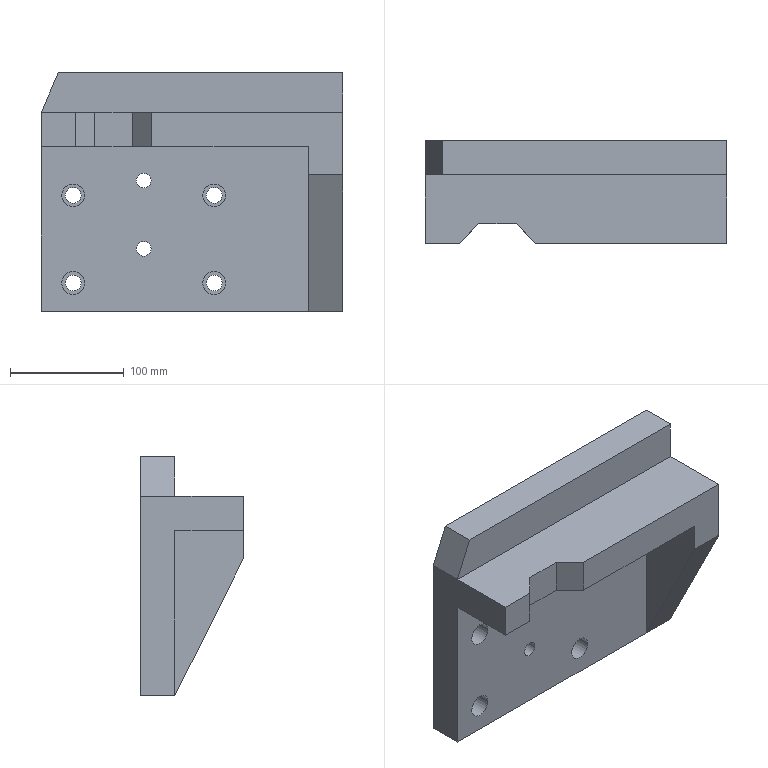Part | NX | features solid 2 | 1 solid | 31 faces | box 265 x 90 x 210 mm | volume 2230075 mm3 | plane 21 | cylinder 10 | commonest cylinder face diameters 14 x4 20 x4 13 x2
STEP:
#1=CARTESIAN_POINT('',(40.,505.,-125.));
#2=VERTEX_POINT('',#1);
#3=CARTESIAN_POINT('',(70.,505.,-125.));
#4=VERTEX_POINT('',#3);
#5=CARTESIAN_POINT('',(40.,505.,-125.));
#6=DIRECTION('',(1.,0.,0.));
#7=VECTOR('',#6,1000.);
#8=LINE('',#5,#7);
#9=EDGE_CURVE('',#2,#4,#8,.T.);
#10=ORIENTED_EDGE('',*,*,#9,.T.);
#11=CARTESIAN_POINT('',(70.,505.,-70.));
#12=VERTEX_POINT('',#11);
#13=CARTESIAN_POINT('',(70.,505.,-70.));
#14=DIRECTION('',(0.,0.,-1.));
#15=VECTOR('',#14,1000.);
#16=LINE('',#13,#15);
#17=EDGE_CURVE('',#12,#4,#16,.T.);
#18=ORIENTED_EDGE('',*,*,#17,.F.);
#19=CARTESIAN_POINT('',(-98.,505.,-70.));
#20=VERTEX_POINT('',#19);
#21=CARTESIAN_POINT('',(-235.,505.,-70.));
#22=DIRECTION('',(-1.,0.,0.));
#23=VECTOR('',#22,1000.);
#24=LINE('',#21,#23);
#25=EDGE_CURVE('',#20,#12,#24,.F.);
#26=ORIENTED_EDGE('',*,*,#25,.F.);
#27=CARTESIAN_POINT('',(-98.,505.,-100.));
#28=VERTEX_POINT('',#27);
#29=CARTESIAN_POINT('',(-98.,505.,-95.974));
#30=DIRECTION('',(0.,0.,-1.));
#31=VECTOR('',#30,1000.);
#32=LINE('',#29,#31);
#33=EDGE_CURVE('',#20,#28,#32,.T.);
#34=ORIENTED_EDGE('',*,*,#33,.T.);
#35=CARTESIAN_POINT('',(40.,505.,-100.));
#36=VERTEX_POINT('',#35);
#37=CARTESIAN_POINT('',(70.,505.,-100.));
#38=DIRECTION('',(-1.,0.,0.));
#39=VECTOR('',#38,1000.);
#40=LINE('',#37,#39);
#41=EDGE_CURVE('',#28,#36,#40,.F.);
#42=ORIENTED_EDGE('',*,*,#41,.T.);
#43=CARTESIAN_POINT('',(40.,505.,-95.974));
#44=DIRECTION('',(0.,0.,-1.));
#45=VECTOR('',#44,1000.);
#46=LINE('',#43,#45);
#47=EDGE_CURVE('',#36,#2,#46,.T.);
#48=ORIENTED_EDGE('',*,*,#47,.T.);
#49=EDGE_LOOP('',(#10,#18,#26,#34,#42,#48));
#50=FACE_BOUND('',#49,.T.);
#51=CARTESIAN_POINT('',(115.,505.,-95.974));
#52=DIRECTION('',(0.,1.,0.));
#53=DIRECTION('',(-1.,0.,0.));
#54=AXIS2_PLACEMENT_3D('',#51,#52,#53);
#55=PLANE('',#54);
#56=ADVANCED_FACE('',(#50),#55,.F.);
#57=CARTESIAN_POINT('',(-50.,595.,-143.));
#58=VERTEX_POINT('',#57);
#59=CARTESIAN_POINT('',(-43.,595.,-143.));
#60=DIRECTION('',(0.,1.,0.));
#61=DIRECTION('',(-1.,0.,0.));
#62=AXIS2_PLACEMENT_3D('',#59,#60,#61);
#63=CIRCLE('',#62,7.);
#64=EDGE_CURVE('',#58,#58,#63,.F.);
#65=ORIENTED_EDGE('',*,*,#64,.T.);
#66=EDGE_LOOP('',(#65));
#67=FACE_BOUND('',#66,.T.);
#68=CARTESIAN_POINT('',(-111.5,595.,-130.));
#69=VERTEX_POINT('',#68);
#70=CARTESIAN_POINT('',(-105.,595.,-130.));
#71=DIRECTION('',(0.,1.,0.));
#72=DIRECTION('',(-1.,0.,0.));
#73=AXIS2_PLACEMENT_3D('',#70,#71,#72);
#74=CIRCLE('',#73,6.5);
#75=EDGE_CURVE('',#69,#69,#74,.T.);
#76=ORIENTED_EDGE('',*,*,#75,.F.);
#77=EDGE_LOOP('',(#76));
#78=FACE_BOUND('',#77,.T.);
#79=CARTESIAN_POINT('',(-50.,595.,-220.));
#80=VERTEX_POINT('',#79);
#81=CARTESIAN_POINT('',(-43.,595.,-220.));
#82=DIRECTION('',(0.,1.,0.));
#83=DIRECTION('',(-1.,0.,0.));
#84=AXIS2_PLACEMENT_3D('',#81,#82,#83);
#85=CIRCLE('',#84,7.);
#86=EDGE_CURVE('',#80,#80,#85,.F.);
#87=ORIENTED_EDGE('',*,*,#86,.T.);
#88=EDGE_LOOP('',(#87));
#89=FACE_BOUND('',#88,.T.);
#90=CARTESIAN_POINT('',(-111.5,595.,-190.));
#91=VERTEX_POINT('',#90);
#92=CARTESIAN_POINT('',(-105.,595.,-190.));
#93=DIRECTION('',(0.,1.,0.));
#94=DIRECTION('',(-1.,0.,0.));
#95=AXIS2_PLACEMENT_3D('',#92,#93,#94);
#96=CIRCLE('',#95,6.5);
#97=EDGE_CURVE('',#91,#91,#96,.T.);
#98=ORIENTED_EDGE('',*,*,#97,.F.);
#99=EDGE_LOOP('',(#98));
#100=FACE_BOUND('',#99,.T.);
#101=CARTESIAN_POINT('',(-174.,595.,-220.));
#102=VERTEX_POINT('',#101);
#103=CARTESIAN_POINT('',(-167.,595.,-220.));
#104=DIRECTION('',(0.,1.,0.));
#105=DIRECTION('',(-1.,0.,0.));
#106=AXIS2_PLACEMENT_3D('',#103,#104,#105);
#107=CIRCLE('',#106,7.);
#108=EDGE_CURVE('',#102,#102,#107,.F.);
#109=ORIENTED_EDGE('',*,*,#108,.T.);
#110=EDGE_LOOP('',(#109));
#111=FACE_BOUND('',#110,.T.);
#112=CARTESIAN_POINT('',(-174.,595.,-143.));
#113=VERTEX_POINT('',#112);
#114=CARTESIAN_POINT('',(-167.,595.,-143.));
#115=DIRECTION('',(0.,1.,0.));
#116=DIRECTION('',(-1.,0.,0.));
#117=AXIS2_PLACEMENT_3D('',#114,#115,#116);
#118=CIRCLE('',#117,7.);
#119=EDGE_CURVE('',#113,#113,#118,.F.);
#120=ORIENTED_EDGE('',*,*,#119,.T.);
#121=EDGE_LOOP('',(#120));
#122=FACE_BOUND('',#121,.T.);
#123=CARTESIAN_POINT('',(-180.,595.,-35.));
#124=VERTEX_POINT('',#123);
#125=CARTESIAN_POINT('',(70.,595.,-35.));
#126=VERTEX_POINT('',#125);
#127=CARTESIAN_POINT('',(-70.,595.,-35.));
#128=DIRECTION('',(-1.,0.,0.));
#129=VECTOR('',#128,1000.);
#130=LINE('',#127,#129);
#131=EDGE_CURVE('',#124,#126,#130,.F.);
#132=ORIENTED_EDGE('',*,*,#131,.T.);
#133=CARTESIAN_POINT('',(70.,595.,-245.));
#134=VERTEX_POINT('',#133);
#135=CARTESIAN_POINT('',(70.,595.,-55.974));
#136=DIRECTION('',(0.,0.,-1.));
#137=VECTOR('',#136,1000.);
#138=LINE('',#135,#137);
#139=EDGE_CURVE('',#126,#134,#138,.T.);
#140=ORIENTED_EDGE('',*,*,#139,.T.);
#141=CARTESIAN_POINT('',(-195.,595.,-245.));
#142=VERTEX_POINT('',#141);
#143=CARTESIAN_POINT('',(-195.,595.,-245.));
#144=DIRECTION('',(-1.,0.,0.));
#145=VECTOR('',#144,1000.);
#146=LINE('',#143,#145);
#147=EDGE_CURVE('',#142,#134,#146,.F.);
#148=ORIENTED_EDGE('',*,*,#147,.F.);
#149=CARTESIAN_POINT('',(-195.,595.,-70.));
#150=VERTEX_POINT('',#149);
#151=CARTESIAN_POINT('',(-195.,595.,-245.));
#152=DIRECTION('',(0.,0.,1.));
#153=VECTOR('',#152,1000.);
#154=LINE('',#151,#153);
#155=EDGE_CURVE('',#150,#142,#154,.F.);
#156=ORIENTED_EDGE('',*,*,#155,.F.);
#157=CARTESIAN_POINT('',(-141.818,595.,54.091));
#158=DIRECTION('',(-0.3939,0.,-0.9191));
#159=VECTOR('',#158,1000.);
#160=LINE('',#157,#159);
#161=EDGE_CURVE('',#150,#124,#160,.F.);
#162=ORIENTED_EDGE('',*,*,#161,.T.);
#163=EDGE_LOOP('',(#132,#140,#148,#156,#162));
#164=FACE_BOUND('',#163,.T.);
#165=CARTESIAN_POINT('',(115.,595.,-55.974));
#166=DIRECTION('',(0.,1.,0.));
#167=DIRECTION('',(-1.,0.,0.));
#168=AXIS2_PLACEMENT_3D('',#165,#166,#167);
#169=PLANE('',#168);
#170=ADVANCED_FACE('',(#67,#78,#89,#100,#111,#122,#164),#169,.T.);
#171=ORIENTED_EDGE('',*,*,#147,.T.);
#172=CARTESIAN_POINT('',(70.,565.,-245.));
#173=VERTEX_POINT('',#172);
#174=CARTESIAN_POINT('',(70.,595.,-245.));
#175=DIRECTION('',(0.,-1.,0.));
#176=VECTOR('',#175,1000.);
#177=LINE('',#174,#176);
#178=EDGE_CURVE('',#134,#173,#177,.T.);
#179=ORIENTED_EDGE('',*,*,#178,.T.);
#180=CARTESIAN_POINT('',(40.,565.,-245.));
#181=VERTEX_POINT('',#180);
#182=CARTESIAN_POINT('',(-195.,565.,-245.));
#183=DIRECTION('',(1.,0.,0.));
#184=VECTOR('',#183,1000.);
#185=LINE('',#182,#184);
#186=EDGE_CURVE('',#181,#173,#185,.T.);
#187=ORIENTED_EDGE('',*,*,#186,.F.);
#188=CARTESIAN_POINT('',(-195.,565.,-245.));
#189=VERTEX_POINT('',#188);
#190=CARTESIAN_POINT('',(-195.,565.,-245.));
#191=DIRECTION('',(-1.,0.,0.));
#192=VECTOR('',#191,1000.);
#193=LINE('',#190,#192);
#194=EDGE_CURVE('',#189,#181,#193,.F.);
#195=ORIENTED_EDGE('',*,*,#194,.F.);
#196=CARTESIAN_POINT('',(-195.,595.,-245.));
#197=DIRECTION('',(0.,-1.,0.));
#198=VECTOR('',#197,1000.);
#199=LINE('',#196,#198);
#200=EDGE_CURVE('',#142,#189,#199,.T.);
#201=ORIENTED_EDGE('',*,*,#200,.F.);
#202=EDGE_LOOP('',(#171,#179,#187,#195,#201));
#203=FACE_BOUND('',#202,.T.);
#204=CARTESIAN_POINT('',(-195.,595.,-245.));
#205=DIRECTION('',(0.,0.,-1.));
#206=DIRECTION('',(0.,-1.,0.));
#207=AXIS2_PLACEMENT_3D('',#204,#205,#206);
#208=PLANE('',#207);
#209=ADVANCED_FACE('',(#203),#208,.T.);
#210=CARTESIAN_POINT('',(-43.,565.,-210.));
#211=VERTEX_POINT('',#210);
#212=CARTESIAN_POINT('',(-43.,565.,-220.));
#213=DIRECTION('',(0.,1.,0.));
#214=DIRECTION('',(0.,0.,1.));
#215=AXIS2_PLACEMENT_3D('',#212,#213,#214);
#216=CIRCLE('',#215,10.);
#217=EDGE_CURVE('',#211,#211,#216,.T.);
#218=ORIENTED_EDGE('',*,*,#217,.T.);
#219=EDGE_LOOP('',(#218));
#220=FACE_BOUND('',#219,.T.);
#221=CARTESIAN_POINT('',(-43.,565.,-133.));
#222=VERTEX_POINT('',#221);
#223=CARTESIAN_POINT('',(-43.,565.,-143.));
#224=DIRECTION('',(0.,1.,0.));
#225=DIRECTION('',(0.,0.,1.));
#226=AXIS2_PLACEMENT_3D('',#223,#224,#225);
#227=CIRCLE('',#226,10.);
#228=EDGE_CURVE('',#222,#222,#227,.T.);
#229=ORIENTED_EDGE('',*,*,#228,.T.);
#230=EDGE_LOOP('',(#229));
#231=FACE_BOUND('',#230,.T.);
#232=CARTESIAN_POINT('',(-167.,565.,-133.));
#233=VERTEX_POINT('',#232);
#234=CARTESIAN_POINT('',(-167.,565.,-143.));
#235=DIRECTION('',(0.,1.,0.));
#236=DIRECTION('',(0.,0.,1.));
#237=AXIS2_PLACEMENT_3D('',#234,#235,#236);
#238=CIRCLE('',#237,10.);
#239=EDGE_CURVE('',#233,#233,#238,.T.);
#240=ORIENTED_EDGE('',*,*,#239,.T.);
#241=EDGE_LOOP('',(#240));
#242=FACE_BOUND('',#241,.T.);
#243=CARTESIAN_POINT('',(-167.,565.,-210.));
#244=VERTEX_POINT('',#243);
#245=CARTESIAN_POINT('',(-167.,565.,-220.));
#246=DIRECTION('',(0.,1.,0.));
#247=DIRECTION('',(0.,0.,1.));
#248=AXIS2_PLACEMENT_3D('',#245,#246,#247);
#249=CIRCLE('',#248,10.);
#250=EDGE_CURVE('',#244,#244,#249,.T.);
#251=ORIENTED_EDGE('',*,*,#250,.T.);
#252=EDGE_LOOP('',(#251));
#253=FACE_BOUND('',#252,.T.);
#254=CARTESIAN_POINT('',(-111.5,565.,-190.));
#255=VERTEX_POINT('',#254);
#256=CARTESIAN_POINT('',(-105.,565.,-190.));
#257=DIRECTION('',(0.,1.,0.));
#258=DIRECTION('',(-1.,0.,0.));
#259=AXIS2_PLACEMENT_3D('',#256,#257,#258);
#260=CIRCLE('',#259,6.5);
#261=EDGE_CURVE('',#255,#255,#260,.T.);
#262=ORIENTED_EDGE('',*,*,#261,.T.);
#263=EDGE_LOOP('',(#262));
#264=FACE_BOUND('',#263,.T.);
#265=CARTESIAN_POINT('',(-111.5,565.,-130.));
#266=VERTEX_POINT('',#265);
#267=CARTESIAN_POINT('',(-105.,565.,-130.));
#268=DIRECTION('',(0.,1.,0.));
#269=DIRECTION('',(-1.,0.,0.));
#270=AXIS2_PLACEMENT_3D('',#267,#268,#269);
#271=CIRCLE('',#270,6.5);
#272=EDGE_CURVE('',#266,#266,#271,.T.);
#273=ORIENTED_EDGE('',*,*,#272,.T.);
#274=EDGE_LOOP('',(#273));
#275=FACE_BOUND('',#274,.T.);
#276=ORIENTED_EDGE('',*,*,#194,.T.);
#277=CARTESIAN_POINT('',(40.,565.,-100.));
#278=VERTEX_POINT('',#277);
#279=CARTESIAN_POINT('',(40.,565.,-55.974));
#280=DIRECTION('',(0.,0.,-1.));
#281=VECTOR('',#280,1000.);
#282=LINE('',#279,#281);
#283=EDGE_CURVE('',#278,#181,#282,.T.);
#284=ORIENTED_EDGE('',*,*,#283,.F.);
#285=CARTESIAN_POINT('',(-195.,565.,-100.));
#286=VERTEX_POINT('',#285);
#287=CARTESIAN_POINT('',(70.,565.,-100.));
#288=DIRECTION('',(-1.,0.,0.));
#289=VECTOR('',#288,1000.);
#290=LINE('',#287,#289);
#291=EDGE_CURVE('',#286,#278,#290,.F.);
#292=ORIENTED_EDGE('',*,*,#291,.F.);
#293=CARTESIAN_POINT('',(-195.,565.,-245.));
#294=DIRECTION('',(0.,0.,1.));
#295=VECTOR('',#294,1000.);
#296=LINE('',#293,#295);
#297=EDGE_CURVE('',#286,#189,#296,.F.);
#298=ORIENTED_EDGE('',*,*,#297,.T.);
#299=EDGE_LOOP('',(#276,#284,#292,#298));
#300=FACE_BOUND('',#299,.T.);
#301=CARTESIAN_POINT('',(115.,565.,-55.974));
#302=DIRECTION('',(0.,1.,0.));
#303=DIRECTION('',(-1.,0.,0.));
#304=AXIS2_PLACEMENT_3D('',#301,#302,#303);
#305=PLANE('',#304);
#306=ADVANCED_FACE('',(#220,#231,#242,#253,#264,#275,#300),#305,.F.);
#307=ORIENTED_EDGE('',*,*,#200,.T.);
#308=ORIENTED_EDGE('',*,*,#297,.F.);
#309=CARTESIAN_POINT('',(-195.,505.,-100.));
#310=VERTEX_POINT('',#309);
#311=CARTESIAN_POINT('',(-195.,575.,-100.));
#312=DIRECTION('',(0.,-1.,0.));
#313=VECTOR('',#312,1000.);
#314=LINE('',#311,#313);
#315=EDGE_CURVE('',#286,#310,#314,.T.);
#316=ORIENTED_EDGE('',*,*,#315,.T.);
#317=CARTESIAN_POINT('',(-195.,505.,-70.));
#318=VERTEX_POINT('',#317);
#319=CARTESIAN_POINT('',(-195.,505.,-245.));
#320=DIRECTION('',(0.,0.,-1.));
#321=VECTOR('',#320,1000.);
#322=LINE('',#319,#321);
#323=EDGE_CURVE('',#318,#310,#322,.T.);
#324=ORIENTED_EDGE('',*,*,#323,.F.);
#325=CARTESIAN_POINT('',(-195.,565.,-70.));
#326=VERTEX_POINT('',#325);
#327=CARTESIAN_POINT('',(-195.,565.,-70.));
#328=DIRECTION('',(0.,-1.,0.));
#329=VECTOR('',#328,1000.);
#330=LINE('',#327,#329);
#331=EDGE_CURVE('',#326,#318,#330,.T.);
#332=ORIENTED_EDGE('',*,*,#331,.F.);
#333=CARTESIAN_POINT('',(-195.,615.,-70.));
#334=DIRECTION('',(0.,-1.,0.));
#335=VECTOR('',#334,1000.);
#336=LINE('',#333,#335);
#337=EDGE_CURVE('',#326,#150,#336,.F.);
#338=ORIENTED_EDGE('',*,*,#337,.T.);
#339=ORIENTED_EDGE('',*,*,#155,.T.);
#340=EDGE_LOOP('',(#307,#308,#316,#324,#332,#338,#339));
#341=FACE_BOUND('',#340,.T.);
#342=CARTESIAN_POINT('',(-195.,615.,-245.));
#343=DIRECTION('',(-1.,0.,0.));
#344=DIRECTION('',(0.,0.,1.));
#345=AXIS2_PLACEMENT_3D('',#342,#343,#344);
#346=PLANE('',#345);
#347=ADVANCED_FACE('',(#341),#346,.T.);
#348=CARTESIAN_POINT('',(-165.,505.,-100.));
#349=VERTEX_POINT('',#348);
#350=CARTESIAN_POINT('',(70.,505.,-100.));
#351=DIRECTION('',(-1.,0.,0.));
#352=VECTOR('',#351,1000.);
#353=LINE('',#350,#352);
#354=EDGE_CURVE('',#310,#349,#353,.F.);
#355=ORIENTED_EDGE('',*,*,#354,.T.);
#356=CARTESIAN_POINT('',(-165.,505.,-70.));
#357=VERTEX_POINT('',#356);
#358=CARTESIAN_POINT('',(-165.,505.,-95.974));
#359=DIRECTION('',(0.,0.,1.));
#360=VECTOR('',#359,1000.);
#361=LINE('',#358,#360);
#362=EDGE_CURVE('',#349,#357,#361,.T.);
#363=ORIENTED_EDGE('',*,*,#362,.T.);
#364=CARTESIAN_POINT('',(-235.,505.,-70.));
#365=DIRECTION('',(-1.,0.,0.));
#366=VECTOR('',#365,1000.);
#367=LINE('',#364,#366);
#368=EDGE_CURVE('',#318,#357,#367,.F.);
#369=ORIENTED_EDGE('',*,*,#368,.F.);
#370=ORIENTED_EDGE('',*,*,#323,.T.);
#371=EDGE_LOOP('',(#355,#363,#369,#370));
#372=FACE_BOUND('',#371,.T.);
#373=CARTESIAN_POINT('',(115.,505.,-95.974));
#374=DIRECTION('',(0.,1.,0.));
#375=DIRECTION('',(-1.,0.,0.));
#376=AXIS2_PLACEMENT_3D('',#373,#374,#375);
#377=PLANE('',#376);
#378=ADVANCED_FACE('',(#372),#377,.F.);
#379=CARTESIAN_POINT('',(-180.,565.,-35.));
#380=VERTEX_POINT('',#379);
#381=CARTESIAN_POINT('',(70.,565.,-35.));
#382=VERTEX_POINT('',#381);
#383=CARTESIAN_POINT('',(-70.,565.,-35.));
#384=DIRECTION('',(-1.,0.,0.));
#385=VECTOR('',#384,1000.);
#386=LINE('',#383,#385);
#387=EDGE_CURVE('',#380,#382,#386,.F.);
#388=ORIENTED_EDGE('',*,*,#387,.F.);
#389=CARTESIAN_POINT('',(-195.,565.,-70.));
#390=DIRECTION('',(0.3939,0.,0.9191));
#391=VECTOR('',#390,1000.);
#392=LINE('',#389,#391);
#393=EDGE_CURVE('',#380,#326,#392,.F.);
#394=ORIENTED_EDGE('',*,*,#393,.T.);
#395=CARTESIAN_POINT('',(70.,565.,-70.));
#396=VERTEX_POINT('',#395);
#397=CARTESIAN_POINT('',(-235.,565.,-70.));
#398=DIRECTION('',(-1.,0.,0.));
#399=VECTOR('',#398,1000.);
#400=LINE('',#397,#399);
#401=EDGE_CURVE('',#326,#396,#400,.F.);
#402=ORIENTED_EDGE('',*,*,#401,.T.);
#403=CARTESIAN_POINT('',(70.,565.,-100.));
#404=DIRECTION('',(0.,0.,1.));
#405=VECTOR('',#404,1000.);
#406=LINE('',#403,#405);
#407=EDGE_CURVE('',#396,#382,#406,.T.);
#408=ORIENTED_EDGE('',*,*,#407,.T.);
#409=EDGE_LOOP('',(#388,#394,#402,#408));
#410=FACE_BOUND('',#409,.T.);
#411=CARTESIAN_POINT('',(115.,565.,-55.974));
#412=DIRECTION('',(0.,1.,0.));
#413=DIRECTION('',(-1.,0.,0.));
#414=AXIS2_PLACEMENT_3D('',#411,#412,#413);
#415=PLANE('',#414);
#416=ADVANCED_FACE('',(#410),#415,.F.);
#417=CARTESIAN_POINT('',(-174.,580.,-220.));
#418=VERTEX_POINT('',#417);
#419=CARTESIAN_POINT('',(-167.,580.,-220.));
#420=DIRECTION('',(0.,1.,0.));
#421=DIRECTION('',(-1.,0.,0.));
#422=AXIS2_PLACEMENT_3D('',#419,#420,#421);
#423=CIRCLE('',#422,7.);
#424=EDGE_CURVE('',#418,#418,#423,.T.);
#425=ORIENTED_EDGE('',*,*,#424,.F.);
#426=EDGE_LOOP('',(#425));
#427=FACE_BOUND('',#426,.T.);
#428=ORIENTED_EDGE('',*,*,#108,.F.);
#429=EDGE_LOOP('',(#428));
#430=FACE_BOUND('',#429,.T.);
#431=CARTESIAN_POINT('',(-167.,695.,-220.));
#432=DIRECTION('',(0.,-1.,0.));
#433=DIRECTION('',(0.,0.,-1.));
#434=AXIS2_PLACEMENT_3D('',#431,#432,#433);
#435=CYLINDRICAL_SURFACE('',#434,7.);
#436=ADVANCED_FACE('',(#427,#430),#435,.F.);
#437=ORIENTED_EDGE('',*,*,#97,.T.);
#438=EDGE_LOOP('',(#437));
#439=FACE_BOUND('',#438,.T.);
#440=ORIENTED_EDGE('',*,*,#261,.F.);
#441=EDGE_LOOP('',(#440));
#442=FACE_BOUND('',#441,.T.);
#443=CARTESIAN_POINT('',(-105.,695.,-190.));
#444=DIRECTION('',(0.,-1.,0.));
#445=DIRECTION('',(0.,0.,-1.));
#446=AXIS2_PLACEMENT_3D('',#443,#444,#445);
#447=CYLINDRICAL_SURFACE('',#446,6.5);
#448=ADVANCED_FACE('',(#439,#442),#447,.F.);
#449=CARTESIAN_POINT('',(-50.,580.,-220.));
#450=VERTEX_POINT('',#449);
#451=CARTESIAN_POINT('',(-43.,580.,-220.));
#452=DIRECTION('',(0.,1.,0.));
#453=DIRECTION('',(-1.,0.,0.));
#454=AXIS2_PLACEMENT_3D('',#451,#452,#453);
#455=CIRCLE('',#454,7.);
#456=EDGE_CURVE('',#450,#450,#455,.T.);
#457=ORIENTED_EDGE('',*,*,#456,.F.);
#458=EDGE_LOOP('',(#457));
#459=FACE_BOUND('',#458,.T.);
#460=ORIENTED_EDGE('',*,*,#86,.F.);
#461=EDGE_LOOP('',(#460));
#462=FACE_BOUND('',#461,.T.);
#463=CARTESIAN_POINT('',(-43.,695.,-220.));
#464=DIRECTION('',(0.,-1.,0.));
#465=DIRECTION('',(0.,0.,-1.));
#466=AXIS2_PLACEMENT_3D('',#463,#464,#465);
#467=CYLINDRICAL_SURFACE('',#466,7.);
#468=ADVANCED_FACE('',(#459,#462),#467,.F.);
#469=CARTESIAN_POINT('',(-174.,580.,-143.));
#470=VERTEX_POINT('',#469);
#471=CARTESIAN_POINT('',(-167.,580.,-143.));
#472=DIRECTION('',(0.,1.,0.));
#473=DIRECTION('',(-1.,0.,0.));
#474=AXIS2_PLACEMENT_3D('',#471,#472,#473);
#475=CIRCLE('',#474,7.);
#476=EDGE_CURVE('',#470,#470,#475,.T.);
#477=ORIENTED_EDGE('',*,*,#476,.F.);
#478=EDGE_LOOP('',(#477));
#479=FACE_BOUND('',#478,.T.);
#480=ORIENTED_EDGE('',*,*,#119,.F.);
#481=EDGE_LOOP('',(#480));
#482=FACE_BOUND('',#481,.T.);
#483=CARTESIAN_POINT('',(-167.,695.,-143.));
#484=DIRECTION('',(0.,-1.,0.));
#485=DIRECTION('',(0.,0.,-1.));
#486=AXIS2_PLACEMENT_3D('',#483,#484,#485);
#487=CYLINDRICAL_SURFACE('',#486,7.);
#488=ADVANCED_FACE('',(#479,#482),#487,.F.);
#489=ORIENTED_EDGE('',*,*,#75,.T.);
#490=EDGE_LOOP('',(#489));
#491=FACE_BOUND('',#490,.T.);
#492=ORIENTED_EDGE('',*,*,#272,.F.);
#493=EDGE_LOOP('',(#492));
#494=FACE_BOUND('',#493,.T.);
#495=CARTESIAN_POINT('',(-105.,695.,-130.));
#496=DIRECTION('',(0.,-1.,0.));
#497=DIRECTION('',(0.,0.,-1.));
#498=AXIS2_PLACEMENT_3D('',#495,#496,#497);
#499=CYLINDRICAL_SURFACE('',#498,6.5);
#500=ADVANCED_FACE('',(#491,#494),#499,.F.);
#501=CARTESIAN_POINT('',(-50.,580.,-143.));
#502=VERTEX_POINT('',#501);
#503=CARTESIAN_POINT('',(-43.,580.,-143.));
#504=DIRECTION('',(0.,1.,0.));
#505=DIRECTION('',(-1.,0.,0.));
#506=AXIS2_PLACEMENT_3D('',#503,#504,#505);
#507=CIRCLE('',#506,7.);
#508=EDGE_CURVE('',#502,#502,#507,.T.);
#509=ORIENTED_EDGE('',*,*,#508,.F.);
#510=EDGE_LOOP('',(#509));
#511=FACE_BOUND('',#510,.T.);
#512=ORIENTED_EDGE('',*,*,#64,.F.);
#513=EDGE_LOOP('',(#512));
#514=FACE_BOUND('',#513,.T.);
#515=CARTESIAN_POINT('',(-43.,695.,-143.));
#516=DIRECTION('',(0.,-1.,0.));
#517=DIRECTION('',(0.,0.,-1.));
#518=AXIS2_PLACEMENT_3D('',#515,#516,#517);
#519=CYLINDRICAL_SURFACE('',#518,7.);
#520=ADVANCED_FACE('',(#511,#514),#519,.F.);
#521=ORIENTED_EDGE('',*,*,#368,.T.);
#522=CARTESIAN_POINT('',(-148.,522.,-70.));
#523=VERTEX_POINT('',#522);
#524=CARTESIAN_POINT('',(-165.,505.,-70.));
#525=DIRECTION('',(0.7071,0.7071,0.));
#526=VECTOR('',#525,1000.);
#527=LINE('',#524,#526);
#528=EDGE_CURVE('',#357,#523,#527,.T.);
#529=ORIENTED_EDGE('',*,*,#528,.T.);
#530=CARTESIAN_POINT('',(-115.,522.,-70.));
#531=VERTEX_POINT('',#530);
#532=CARTESIAN_POINT('',(-235.,522.,-70.));
#533=DIRECTION('',(1.,0.,0.));
#534=VECTOR('',#533,1000.);
#535=LINE('',#532,#534);
#536=EDGE_CURVE('',#531,#523,#535,.F.);
#537=ORIENTED_EDGE('',*,*,#536,.F.);
#538=CARTESIAN_POINT('',(-196.5,603.5,-70.));
#539=DIRECTION('',(-0.7071,0.7071,0.));
#540=VECTOR('',#539,1000.);
#541=LINE('',#538,#540);
#542=EDGE_CURVE('',#531,#20,#541,.F.);
#543=ORIENTED_EDGE('',*,*,#542,.T.);
#544=ORIENTED_EDGE('',*,*,#25,.T.);
#545=CARTESIAN_POINT('',(70.,565.,-70.));
#546=DIRECTION('',(0.,1.,0.));
#547=VECTOR('',#546,1000.);
#548=LINE('',#545,#547);
#549=EDGE_CURVE('',#396,#12,#548,.F.);
#550=ORIENTED_EDGE('',*,*,#549,.F.);
#551=ORIENTED_EDGE('',*,*,#401,.F.);
#552=ORIENTED_EDGE('',*,*,#331,.T.);
#553=EDGE_LOOP('',(#521,#529,#537,#543,#544,#550,#551,#552));
#554=FACE_BOUND('',#553,.T.);
#555=CARTESIAN_POINT('',(-235.,565.,-70.));
#556=DIRECTION('',(0.,0.,1.));
#557=DIRECTION('',(1.,0.,0.));
#558=AXIS2_PLACEMENT_3D('',#555,#556,#557);
#559=PLANE('',#558);
#560=ADVANCED_FACE('',(#554),#559,.T.);
#561=ORIENTED_EDGE('',*,*,#17,.T.);
#562=CARTESIAN_POINT('',(70.,505.,-125.));
#563=DIRECTION('',(0.,-0.4472,0.8944));
#564=VECTOR('',#563,1000.);
#565=LINE('',#562,#564);
#566=EDGE_CURVE('',#173,#4,#565,.T.);
#567=ORIENTED_EDGE('',*,*,#566,.F.);
#568=ORIENTED_EDGE('',*,*,#178,.F.);
#569=ORIENTED_EDGE('',*,*,#139,.F.);
#570=CARTESIAN_POINT('',(70.,670.,-35.));
#571=DIRECTION('',(0.,1.,0.));
#572=VECTOR('',#571,1000.);
#573=LINE('',#570,#572);
#574=EDGE_CURVE('',#382,#126,#573,.T.);
#575=ORIENTED_EDGE('',*,*,#574,.F.);
#576=ORIENTED_EDGE('',*,*,#407,.F.);
#577=ORIENTED_EDGE('',*,*,#549,.T.);
#578=EDGE_LOOP('',(#561,#567,#568,#569,#575,#576,#577));
#579=FACE_BOUND('',#578,.T.);
#580=CARTESIAN_POINT('',(70.,510.,62.212));
#581=DIRECTION('',(1.,0.,0.));
#582=DIRECTION('',(0.,0.,-1.));
#583=AXIS2_PLACEMENT_3D('',#580,#581,#582);
#584=PLANE('',#583);
#585=ADVANCED_FACE('',(#579),#584,.T.);
#586=ORIENTED_EDGE('',*,*,#131,.F.);
#587=CARTESIAN_POINT('',(-180.,670.,-35.));
#588=DIRECTION('',(0.,1.,0.));
#589=VECTOR('',#588,1000.);
#590=LINE('',#587,#589);
#591=EDGE_CURVE('',#124,#380,#590,.F.);
#592=ORIENTED_EDGE('',*,*,#591,.T.);
#593=ORIENTED_EDGE('',*,*,#387,.T.);
#594=ORIENTED_EDGE('',*,*,#574,.T.);
#595=EDGE_LOOP('',(#586,#592,#593,#594));
#596=FACE_BOUND('',#595,.T.);
#597=CARTESIAN_POINT('',(-70.,670.,-35.));
#598=DIRECTION('',(0.,0.,1.));
#599=DIRECTION('',(0.,-1.,0.));
#600=AXIS2_PLACEMENT_3D('',#597,#598,#599);
#601=PLANE('',#600);
#602=ADVANCED_FACE('',(#596),#601,.T.);
#603=ORIENTED_EDGE('',*,*,#393,.F.);
#604=ORIENTED_EDGE('',*,*,#591,.F.);
#605=ORIENTED_EDGE('',*,*,#161,.F.);
#606=ORIENTED_EDGE('',*,*,#337,.F.);
#607=EDGE_LOOP('',(#603,#604,#605,#606));
#608=FACE_BOUND('',#607,.T.);
#609=CARTESIAN_POINT('',(-195.,615.,-70.));
#610=DIRECTION('',(0.9191,0.,-0.3939));
#611=DIRECTION('',(-0.3939,0.,-0.9191));
#612=AXIS2_PLACEMENT_3D('',#609,#610,#611);
#613=PLANE('',#612);
#614=ADVANCED_FACE('',(#608),#613,.F.);
#615=ORIENTED_EDGE('',*,*,#47,.F.);
#616=CARTESIAN_POINT('',(40.,575.,-100.));
#617=DIRECTION('',(0.,1.,0.));
#618=VECTOR('',#617,1000.);
#619=LINE('',#616,#618);
#620=EDGE_CURVE('',#278,#36,#619,.F.);
#621=ORIENTED_EDGE('',*,*,#620,.F.);
#622=ORIENTED_EDGE('',*,*,#283,.T.);
#623=CARTESIAN_POINT('',(40.,505.,-125.));
#624=DIRECTION('',(0.,-0.4472,0.8944));
#625=VECTOR('',#624,1000.);
#626=LINE('',#623,#625);
#627=EDGE_CURVE('',#181,#2,#626,.T.);
#628=ORIENTED_EDGE('',*,*,#627,.T.);
#629=EDGE_LOOP('',(#615,#621,#622,#628));
#630=FACE_BOUND('',#629,.T.);
#631=CARTESIAN_POINT('',(40.,575.,-100.));
#632=DIRECTION('',(1.,0.,0.));
#633=DIRECTION('',(0.,0.,-1.));
#634=AXIS2_PLACEMENT_3D('',#631,#632,#633);
#635=PLANE('',#634);
#636=ADVANCED_FACE('',(#630),#635,.F.);
#637=CARTESIAN_POINT('',(-115.,522.,-100.));
#638=VERTEX_POINT('',#637);
#639=CARTESIAN_POINT('',(-148.,522.,-100.));
#640=VERTEX_POINT('',#639);
#641=CARTESIAN_POINT('',(70.,522.,-100.));
#642=DIRECTION('',(1.,0.,0.));
#643=VECTOR('',#642,1000.);
#644=LINE('',#641,#643);
#645=EDGE_CURVE('',#638,#640,#644,.F.);
#646=ORIENTED_EDGE('',*,*,#645,.T.);
#647=CARTESIAN_POINT('',(-12.5,657.5,-100.));
#648=DIRECTION('',(-0.7071,-0.7071,0.));
#649=VECTOR('',#648,1000.);
#650=LINE('',#647,#649);
#651=EDGE_CURVE('',#640,#349,#650,.T.);
#652=ORIENTED_EDGE('',*,*,#651,.T.);
#653=ORIENTED_EDGE('',*,*,#354,.F.);
#654=ORIENTED_EDGE('',*,*,#315,.F.);
#655=ORIENTED_EDGE('',*,*,#291,.T.);
#656=ORIENTED_EDGE('',*,*,#620,.T.);
#657=ORIENTED_EDGE('',*,*,#41,.F.);
#658=CARTESIAN_POINT('',(-49.,456.,-100.));
#659=DIRECTION('',(-0.7071,0.7071,0.));
#660=VECTOR('',#659,1000.);
#661=LINE('',#658,#660);
#662=EDGE_CURVE('',#638,#28,#661,.F.);
#663=ORIENTED_EDGE('',*,*,#662,.F.);
#664=EDGE_LOOP('',(#646,#652,#653,#654,#655,#656,#657,#663));
#665=FACE_BOUND('',#664,.T.);
#666=CARTESIAN_POINT('',(70.,575.,-100.));
#667=DIRECTION('',(0.,0.,1.));
#668=DIRECTION('',(0.,-1.,0.));
#669=AXIS2_PLACEMENT_3D('',#666,#667,#668);
#670=PLANE('',#669);
#671=ADVANCED_FACE('',(#665),#670,.F.);
#672=CARTESIAN_POINT('',(-167.,580.,-210.));
#673=VERTEX_POINT('',#672);
#674=CARTESIAN_POINT('',(-167.,580.,-220.));
#675=DIRECTION('',(0.,1.,0.));
#676=DIRECTION('',(0.,0.,1.));
#677=AXIS2_PLACEMENT_3D('',#674,#675,#676);
#678=CIRCLE('',#677,10.);
#679=EDGE_CURVE('',#673,#673,#678,.T.);
#680=ORIENTED_EDGE('',*,*,#679,.T.);
#681=EDGE_LOOP('',(#680));
#682=FACE_BOUND('',#681,.T.);
#683=ORIENTED_EDGE('',*,*,#250,.F.);
#684=EDGE_LOOP('',(#683));
#685=FACE_BOUND('',#684,.T.);
#686=CARTESIAN_POINT('',(-167.,565.,-220.));
#687=DIRECTION('',(0.,1.,0.));
#688=DIRECTION('',(0.,0.,1.));
#689=AXIS2_PLACEMENT_3D('',#686,#687,#688);
#690=CYLINDRICAL_SURFACE('',#689,10.);
#691=ADVANCED_FACE('',(#682,#685),#690,.F.);
#692=ORIENTED_EDGE('',*,*,#679,.F.);
#693=EDGE_LOOP('',(#692));
#694=FACE_BOUND('',#693,.T.);
#695=ORIENTED_EDGE('',*,*,#424,.T.);
#696=EDGE_LOOP('',(#695));
#697=FACE_BOUND('',#696,.T.);
#698=CARTESIAN_POINT('',(-167.,580.,-220.));
#699=DIRECTION('',(0.,-1.,0.));
#700=DIRECTION('',(0.,0.,-1.));
#701=AXIS2_PLACEMENT_3D('',#698,#699,#700);
#702=PLANE('',#701);
#703=ADVANCED_FACE('',(#694,#697),#702,.T.);
#704=CARTESIAN_POINT('',(-167.,580.,-133.));
#705=VERTEX_POINT('',#704);
#706=CARTESIAN_POINT('',(-167.,580.,-143.));
#707=DIRECTION('',(0.,1.,0.));
#708=DIRECTION('',(0.,0.,1.));
#709=AXIS2_PLACEMENT_3D('',#706,#707,#708);
#710=CIRCLE('',#709,10.);
#711=EDGE_CURVE('',#705,#705,#710,.T.);
#712=ORIENTED_EDGE('',*,*,#711,.T.);
#713=EDGE_LOOP('',(#712));
#714=FACE_BOUND('',#713,.T.);
#715=ORIENTED_EDGE('',*,*,#239,.F.);
#716=EDGE_LOOP('',(#715));
#717=FACE_BOUND('',#716,.T.);
#718=CARTESIAN_POINT('',(-167.,565.,-143.));
#719=DIRECTION('',(0.,1.,0.));
#720=DIRECTION('',(0.,0.,1.));
#721=AXIS2_PLACEMENT_3D('',#718,#719,#720);
#722=CYLINDRICAL_SURFACE('',#721,10.);
#723=ADVANCED_FACE('',(#714,#717),#722,.F.);
#724=ORIENTED_EDGE('',*,*,#711,.F.);
#725=EDGE_LOOP('',(#724));
#726=FACE_BOUND('',#725,.T.);
#727=ORIENTED_EDGE('',*,*,#476,.T.);
#728=EDGE_LOOP('',(#727));
#729=FACE_BOUND('',#728,.T.);
#730=CARTESIAN_POINT('',(-167.,580.,-143.));
#731=DIRECTION('',(0.,-1.,0.));
#732=DIRECTION('',(0.,0.,-1.));
#733=AXIS2_PLACEMENT_3D('',#730,#731,#732);
#734=PLANE('',#733);
#735=ADVANCED_FACE('',(#726,#729),#734,.T.);
#736=CARTESIAN_POINT('',(-43.,580.,-133.));
#737=VERTEX_POINT('',#736);
#738=CARTESIAN_POINT('',(-43.,580.,-143.));
#739=DIRECTION('',(0.,1.,0.));
#740=DIRECTION('',(0.,0.,1.));
#741=AXIS2_PLACEMENT_3D('',#738,#739,#740);
#742=CIRCLE('',#741,10.);
#743=EDGE_CURVE('',#737,#737,#742,.T.);
#744=ORIENTED_EDGE('',*,*,#743,.T.);
#745=EDGE_LOOP('',(#744));
#746=FACE_BOUND('',#745,.T.);
#747=ORIENTED_EDGE('',*,*,#228,.F.);
#748=EDGE_LOOP('',(#747));
#749=FACE_BOUND('',#748,.T.);
#750=CARTESIAN_POINT('',(-43.,565.,-143.));
#751=DIRECTION('',(0.,1.,0.));
#752=DIRECTION('',(0.,0.,1.));
#753=AXIS2_PLACEMENT_3D('',#750,#751,#752);
#754=CYLINDRICAL_SURFACE('',#753,10.);
#755=ADVANCED_FACE('',(#746,#749),#754,.F.);
#756=ORIENTED_EDGE('',*,*,#743,.F.);
#757=EDGE_LOOP('',(#756));
#758=FACE_BOUND('',#757,.T.);
#759=ORIENTED_EDGE('',*,*,#508,.T.);
#760=EDGE_LOOP('',(#759));
#761=FACE_BOUND('',#760,.T.);
#762=CARTESIAN_POINT('',(-43.,580.,-143.));
#763=DIRECTION('',(0.,-1.,0.));
#764=DIRECTION('',(0.,0.,-1.));
#765=AXIS2_PLACEMENT_3D('',#762,#763,#764);
#766=PLANE('',#765);
#767=ADVANCED_FACE('',(#758,#761),#766,.T.);
#768=CARTESIAN_POINT('',(-43.,580.,-210.));
#769=VERTEX_POINT('',#768);
#770=CARTESIAN_POINT('',(-43.,580.,-220.));
#771=DIRECTION('',(0.,1.,0.));
#772=DIRECTION('',(0.,0.,1.));
#773=AXIS2_PLACEMENT_3D('',#770,#771,#772);
#774=CIRCLE('',#773,10.);
#775=EDGE_CURVE('',#769,#769,#774,.T.);
#776=ORIENTED_EDGE('',*,*,#775,.T.);
#777=EDGE_LOOP('',(#776));
#778=FACE_BOUND('',#777,.T.);
#779=ORIENTED_EDGE('',*,*,#217,.F.);
#780=EDGE_LOOP('',(#779));
#781=FACE_BOUND('',#780,.T.);
#782=CARTESIAN_POINT('',(-43.,565.,-220.));
#783=DIRECTION('',(0.,1.,0.));
#784=DIRECTION('',(0.,0.,1.));
#785=AXIS2_PLACEMENT_3D('',#782,#783,#784);
#786=CYLINDRICAL_SURFACE('',#785,10.);
#787=ADVANCED_FACE('',(#778,#781),#786,.F.);
#788=ORIENTED_EDGE('',*,*,#775,.F.);
#789=EDGE_LOOP('',(#788));
#790=FACE_BOUND('',#789,.T.);
#791=ORIENTED_EDGE('',*,*,#456,.T.);
#792=EDGE_LOOP('',(#791));
#793=FACE_BOUND('',#792,.T.);
#794=CARTESIAN_POINT('',(-43.,580.,-220.));
#795=DIRECTION('',(0.,-1.,0.));
#796=DIRECTION('',(0.,0.,-1.));
#797=AXIS2_PLACEMENT_3D('',#794,#795,#796);
#798=PLANE('',#797);
#799=ADVANCED_FACE('',(#790,#793),#798,.T.);
#800=CARTESIAN_POINT('',(-115.,522.,-55.));
#801=DIRECTION('',(0.,0.,-1.));
#802=VECTOR('',#801,1000.);
#803=LINE('',#800,#802);
#804=EDGE_CURVE('',#531,#638,#803,.T.);
#805=ORIENTED_EDGE('',*,*,#804,.T.);
#806=ORIENTED_EDGE('',*,*,#662,.T.);
#807=ORIENTED_EDGE('',*,*,#33,.F.);
#808=ORIENTED_EDGE('',*,*,#542,.F.);
#809=EDGE_LOOP('',(#805,#806,#807,#808));
#810=FACE_BOUND('',#809,.T.);
#811=CARTESIAN_POINT('',(-115.,522.,-55.));
#812=DIRECTION('',(0.7071,0.7071,0.));
#813=DIRECTION('',(-0.7071,0.7071,0.));
#814=AXIS2_PLACEMENT_3D('',#811,#812,#813);
#815=PLANE('',#814);
#816=ADVANCED_FACE('',(#810),#815,.F.);
#817=ORIENTED_EDGE('',*,*,#536,.T.);
#818=CARTESIAN_POINT('',(-148.,522.,-95.974));
#819=DIRECTION('',(0.,0.,1.));
#820=VECTOR('',#819,1000.);
#821=LINE('',#818,#820);
#822=EDGE_CURVE('',#523,#640,#821,.F.);
#823=ORIENTED_EDGE('',*,*,#822,.T.);
#824=ORIENTED_EDGE('',*,*,#645,.F.);
#825=ORIENTED_EDGE('',*,*,#804,.F.);
#826=EDGE_LOOP('',(#817,#823,#824,#825));
#827=FACE_BOUND('',#826,.T.);
#828=CARTESIAN_POINT('',(-115.,522.,-55.));
#829=DIRECTION('',(0.,-1.,0.));
#830=DIRECTION('',(0.,0.,1.));
#831=AXIS2_PLACEMENT_3D('',#828,#829,#830);
#832=PLANE('',#831);
#833=ADVANCED_FACE('',(#827),#832,.T.);
#834=ORIENTED_EDGE('',*,*,#651,.F.);
#835=ORIENTED_EDGE('',*,*,#822,.F.);
#836=ORIENTED_EDGE('',*,*,#528,.F.);
#837=ORIENTED_EDGE('',*,*,#362,.F.);
#838=EDGE_LOOP('',(#834,#835,#836,#837));
#839=FACE_BOUND('',#838,.T.);
#840=CARTESIAN_POINT('',(-165.,505.,-95.974));
#841=DIRECTION('',(-0.7071,0.7071,0.));
#842=DIRECTION('',(-0.7071,-0.7071,0.));
#843=AXIS2_PLACEMENT_3D('',#840,#841,#842);
#844=PLANE('',#843);
#845=ADVANCED_FACE('',(#839),#844,.F.);
#846=ORIENTED_EDGE('',*,*,#186,.T.);
#847=ORIENTED_EDGE('',*,*,#566,.T.);
#848=ORIENTED_EDGE('',*,*,#9,.F.);
#849=ORIENTED_EDGE('',*,*,#627,.F.);
#850=EDGE_LOOP('',(#846,#847,#848,#849));
#851=FACE_BOUND('',#850,.T.);
#852=CARTESIAN_POINT('',(40.,565.,-245.));
#853=DIRECTION('',(0.,-0.8944,-0.4472));
#854=DIRECTION('',(0.,0.4472,-0.8944));
#855=AXIS2_PLACEMENT_3D('',#852,#853,#854);
#856=PLANE('',#855);
#857=ADVANCED_FACE('',(#851),#856,.T.);
#858=CLOSED_SHELL('',(#56,#170,#209,#306,#347,#378,#416,#436,#448,#468,#488,#500,#520,#560,#585,#602,#614,#636,#671,#691,#703,#723,#735,#755,#767,#787,#799,#816,#833,#845,#857));
#859=MANIFOLD_SOLID_BREP('',#858);
#860=(LENGTH_UNIT()NAMED_UNIT(*)SI_UNIT(.MILLI.,.METRE.));
#861=UNCERTAINTY_MEASURE_WITH_UNIT(LENGTH_MEASURE(0.00001),#860,'','');
#862=(NAMED_UNIT(*)PLANE_ANGLE_UNIT()SI_UNIT($,.RADIAN.));
#863=(NAMED_UNIT(*)SI_UNIT($,.STERADIAN.)SOLID_ANGLE_UNIT());
#864=(GEOMETRIC_REPRESENTATION_CONTEXT(3)GLOBAL_UNCERTAINTY_ASSIGNED_CONTEXT((#861))GLOBAL_UNIT_ASSIGNED_CONTEXT((#860,#862,#863))REPRESENTATION_CONTEXT('',''));
#865=ADVANCED_BREP_SHAPE_REPRESENTATION('',(#859),#864);